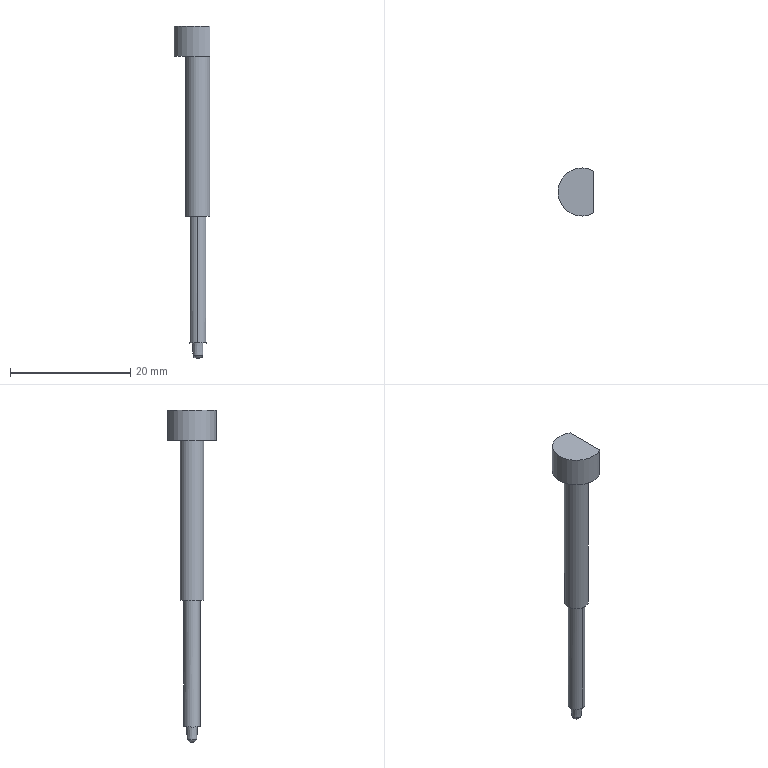Part | NX | features solid 2 | 1 solid | 12 faces | box 6 x 8 x 55.164 mm | volume 670.32 mm3 | plane 5 | cylinder 4 | cone 2 | torus 1 | commonest cylinder face diameters 2.785 x2 4 x1 8 x1
STEP:
#1=CARTESIAN_POINT('',(2.,37.688,65.5));
#2=VERTEX_POINT('',#1);
#3=CARTESIAN_POINT('',(0.,37.688,65.5));
#4=DIRECTION('',(0.,0.,-1.));
#5=DIRECTION('',(-1.,0.,0.));
#6=AXIS2_PLACEMENT_3D('',#3,#4,#5);
#7=CIRCLE('',#6,2.);
#8=EDGE_CURVE('',#2,#2,#7,.F.);
#9=ORIENTED_EDGE('',*,*,#8,.F.);
#10=EDGE_LOOP('',(#9));
#11=FACE_BOUND('',#10,.T.);
#12=CARTESIAN_POINT('',(-2.,37.688,38.875));
#13=VERTEX_POINT('',#12);
#14=CARTESIAN_POINT('',(0.,37.688,38.875));
#15=DIRECTION('',(0.,0.,-1.));
#16=DIRECTION('',(-1.,0.,0.));
#17=AXIS2_PLACEMENT_3D('',#14,#15,#16);
#18=CIRCLE('',#17,2.);
#19=EDGE_CURVE('',#13,#13,#18,.F.);
#20=ORIENTED_EDGE('',*,*,#19,.T.);
#21=EDGE_LOOP('',(#20));
#22=FACE_BOUND('',#21,.T.);
#23=CARTESIAN_POINT('',(0.,37.688,117.875));
#24=DIRECTION('',(0.,0.,-1.));
#25=DIRECTION('',(-1.,0.,0.));
#26=AXIS2_PLACEMENT_3D('',#23,#24,#25);
#27=CYLINDRICAL_SURFACE('',#26,2.);
#28=ADVANCED_FACE('',(#11,#22),#27,.T.);
#29=CARTESIAN_POINT('',(2.,34.223,65.5));
#30=VERTEX_POINT('',#29);
#31=CARTESIAN_POINT('',(2.,41.152,65.5));
#32=VERTEX_POINT('',#31);
#33=CARTESIAN_POINT('',(0.,37.688,65.5));
#34=DIRECTION('',(0.,0.,-1.));
#35=DIRECTION('',(-1.,0.,0.));
#36=AXIS2_PLACEMENT_3D('',#33,#34,#35);
#37=CIRCLE('',#36,4.);
#38=EDGE_CURVE('',#30,#32,#37,.T.);
#39=ORIENTED_EDGE('',*,*,#38,.F.);
#40=CARTESIAN_POINT('',(2.,34.223,70.5));
#41=VERTEX_POINT('',#40);
#42=CARTESIAN_POINT('',(2.,34.223,66.5));
#43=DIRECTION('',(0.,0.,1.));
#44=VECTOR('',#43,1000.);
#45=LINE('',#42,#44);
#46=EDGE_CURVE('',#41,#30,#45,.F.);
#47=ORIENTED_EDGE('',*,*,#46,.F.);
#48=CARTESIAN_POINT('',(2.,41.152,70.5));
#49=VERTEX_POINT('',#48);
#50=CARTESIAN_POINT('',(0.,37.688,70.5));
#51=DIRECTION('',(0.,0.,1.));
#52=DIRECTION('',(1.,0.,0.));
#53=AXIS2_PLACEMENT_3D('',#50,#51,#52);
#54=CIRCLE('',#53,4.);
#55=EDGE_CURVE('',#41,#49,#54,.F.);
#56=ORIENTED_EDGE('',*,*,#55,.T.);
#57=CARTESIAN_POINT('',(2.,41.152,66.5));
#58=DIRECTION('',(0.,0.,1.));
#59=VECTOR('',#58,1000.);
#60=LINE('',#57,#59);
#61=EDGE_CURVE('',#32,#49,#60,.T.);
#62=ORIENTED_EDGE('',*,*,#61,.F.);
#63=EDGE_LOOP('',(#39,#47,#56,#62));
#64=FACE_BOUND('',#63,.T.);
#65=CARTESIAN_POINT('',(0.,37.688,66.5));
#66=DIRECTION('',(0.,0.,1.));
#67=DIRECTION('',(1.,0.,0.));
#68=AXIS2_PLACEMENT_3D('',#65,#66,#67);
#69=CYLINDRICAL_SURFACE('',#68,4.);
#70=ADVANCED_FACE('',(#64),#69,.T.);
#71=CARTESIAN_POINT('',(2.,37.688,65.5));
#72=DIRECTION('',(0.,-1.,0.));
#73=VECTOR('',#72,1000.);
#74=LINE('',#71,#73);
#75=EDGE_CURVE('',#2,#32,#74,.F.);
#76=ORIENTED_EDGE('',*,*,#75,.F.);
#77=ORIENTED_EDGE('',*,*,#8,.T.);
#78=CARTESIAN_POINT('',(2.,37.688,65.5));
#79=DIRECTION('',(0.,-1.,0.));
#80=VECTOR('',#79,1000.);
#81=LINE('',#78,#80);
#82=EDGE_CURVE('',#30,#2,#81,.F.);
#83=ORIENTED_EDGE('',*,*,#82,.F.);
#84=ORIENTED_EDGE('',*,*,#38,.T.);
#85=EDGE_LOOP('',(#76,#77,#83,#84));
#86=FACE_BOUND('',#85,.T.);
#87=CARTESIAN_POINT('',(0.,37.688,65.5));
#88=DIRECTION('',(0.,0.,-1.));
#89=DIRECTION('',(-1.,0.,0.));
#90=AXIS2_PLACEMENT_3D('',#87,#88,#89);
#91=PLANE('',#90);
#92=ADVANCED_FACE('',(#86),#91,.T.);
#93=CARTESIAN_POINT('',(2.,0.,70.5));
#94=DIRECTION('',(0.,1.,0.));
#95=VECTOR('',#94,1000.);
#96=LINE('',#93,#95);
#97=EDGE_CURVE('',#49,#41,#96,.F.);
#98=ORIENTED_EDGE('',*,*,#97,.F.);
#99=ORIENTED_EDGE('',*,*,#55,.F.);
#100=EDGE_LOOP('',(#98,#99));
#101=FACE_BOUND('',#100,.T.);
#102=CARTESIAN_POINT('',(0.,0.,70.5));
#103=DIRECTION('',(0.,0.,1.));
#104=DIRECTION('',(1.,0.,0.));
#105=AXIS2_PLACEMENT_3D('',#102,#103,#104);
#106=PLANE('',#105);
#107=ADVANCED_FACE('',(#101),#106,.T.);
#108=CARTESIAN_POINT('',(0.,36.295,17.916));
#109=VERTEX_POINT('',#108);
#110=CARTESIAN_POINT('',(0.,39.08,17.94));
#111=VERTEX_POINT('',#110);
#112=CARTESIAN_POINT('',(0.,36.295,17.916));
#113=CARTESIAN_POINT('',(0.3656,36.295,17.916));
#114=CARTESIAN_POINT('',(1.09,36.596,17.866));
#115=CARTESIAN_POINT('',(1.544,37.687,17.795));
#116=CARTESIAN_POINT('',(1.09,38.779,17.885));
#117=CARTESIAN_POINT('',(0.3667,39.08,17.94));
#118=CARTESIAN_POINT('',(0.,39.08,17.94));
#119=B_SPLINE_CURVE_WITH_KNOTS('',3,(#112,#113,#114,#115,#116,#117,#118),.UNSPECIFIED.,.F.,.F.,(4,1,1,1,4),(0.00007924,0.001169,0.002259,0.003349,0.004439),.UNSPECIFIED.);
#120=EDGE_CURVE('',#109,#111,#119,.T.);
#121=ORIENTED_EDGE('',*,*,#120,.T.);
#122=CARTESIAN_POINT('',(0.,39.08,38.875));
#123=VERTEX_POINT('',#122);
#124=CARTESIAN_POINT('',(0.,39.08,38.875));
#125=DIRECTION('',(0.,0.,-1.));
#126=VECTOR('',#125,1000.);
#127=LINE('',#124,#126);
#128=EDGE_CURVE('',#111,#123,#127,.F.);
#129=ORIENTED_EDGE('',*,*,#128,.T.);
#130=CARTESIAN_POINT('',(0.,36.295,38.875));
#131=VERTEX_POINT('',#130);
#132=CARTESIAN_POINT('',(0.,37.688,38.875));
#133=DIRECTION('',(0.,0.,1.));
#134=DIRECTION('',(0.,-1.,0.));
#135=AXIS2_PLACEMENT_3D('',#132,#133,#134);
#136=CIRCLE('',#135,1.393);
#137=EDGE_CURVE('',#123,#131,#136,.F.);
#138=ORIENTED_EDGE('',*,*,#137,.T.);
#139=CARTESIAN_POINT('',(0.,36.295,38.875));
#140=DIRECTION('',(0.,0.,-1.));
#141=VECTOR('',#140,1000.);
#142=LINE('',#139,#141);
#143=EDGE_CURVE('',#131,#109,#142,.T.);
#144=ORIENTED_EDGE('',*,*,#143,.T.);
#145=EDGE_LOOP('',(#121,#129,#138,#144));
#146=FACE_BOUND('',#145,.T.);
#147=CARTESIAN_POINT('',(0.,37.688,38.875));
#148=DIRECTION('',(0.,0.,1.));
#149=DIRECTION('',(0.,1.,0.));
#150=AXIS2_PLACEMENT_3D('',#147,#148,#149);
#151=CYLINDRICAL_SURFACE('',#150,1.393);
#152=ADVANCED_FACE('',(#146),#151,.T.);
#153=CARTESIAN_POINT('',(0.,39.08,17.94));
#154=CARTESIAN_POINT('',(-0.3656,39.08,17.94));
#155=CARTESIAN_POINT('',(-1.089,38.779,17.885));
#156=CARTESIAN_POINT('',(-1.544,37.69,17.795));
#157=CARTESIAN_POINT('',(-1.091,36.596,17.866));
#158=CARTESIAN_POINT('',(-0.3667,36.295,17.916));
#159=CARTESIAN_POINT('',(0.,36.295,17.916));
#160=B_SPLINE_CURVE_WITH_KNOTS('',3,(#153,#154,#155,#156,#157,#158,#159),.UNSPECIFIED.,.F.,.F.,(4,1,1,1,4),(0.00007934,0.001169,0.002259,0.003349,0.004439),.UNSPECIFIED.);
#161=EDGE_CURVE('',#111,#109,#160,.T.);
#162=ORIENTED_EDGE('',*,*,#161,.T.);
#163=ORIENTED_EDGE('',*,*,#143,.F.);
#164=CARTESIAN_POINT('',(0.,37.688,38.875));
#165=DIRECTION('',(0.,0.,1.));
#166=DIRECTION('',(0.,1.,0.));
#167=AXIS2_PLACEMENT_3D('',#164,#165,#166);
#168=CIRCLE('',#167,1.393);
#169=EDGE_CURVE('',#131,#123,#168,.F.);
#170=ORIENTED_EDGE('',*,*,#169,.T.);
#171=ORIENTED_EDGE('',*,*,#128,.F.);
#172=EDGE_LOOP('',(#162,#163,#170,#171));
#173=FACE_BOUND('',#172,.T.);
#174=CARTESIAN_POINT('',(0.,37.688,38.875));
#175=DIRECTION('',(0.,0.,1.));
#176=DIRECTION('',(0.,1.,0.));
#177=AXIS2_PLACEMENT_3D('',#174,#175,#176);
#178=CYLINDRICAL_SURFACE('',#177,1.393);
#179=ADVANCED_FACE('',(#173),#178,.T.);
#180=ORIENTED_EDGE('',*,*,#19,.F.);
#181=EDGE_LOOP('',(#180));
#182=FACE_BOUND('',#181,.T.);
#183=ORIENTED_EDGE('',*,*,#169,.F.);
#184=ORIENTED_EDGE('',*,*,#137,.F.);
#185=EDGE_LOOP('',(#183,#184));
#186=FACE_BOUND('',#185,.T.);
#187=CARTESIAN_POINT('',(0.,37.688,38.875));
#188=DIRECTION('',(0.,0.,-1.));
#189=DIRECTION('',(0.,-1.,0.));
#190=AXIS2_PLACEMENT_3D('',#187,#188,#189);
#191=PLANE('',#190);
#192=ADVANCED_FACE('',(#182,#186),#191,.T.);
#193=CARTESIAN_POINT('',(-0.3071,37.688,15.336));
#194=VERTEX_POINT('',#193);
#195=CARTESIAN_POINT('',(0.,37.688,15.336));
#196=DIRECTION('',(0.,0.,-1.));
#197=DIRECTION('',(-1.,0.,0.));
#198=AXIS2_PLACEMENT_3D('',#195,#196,#197);
#199=CIRCLE('',#198,0.3071);
#200=EDGE_CURVE('',#194,#194,#199,.T.);
#201=ORIENTED_EDGE('',*,*,#200,.T.);
#202=EDGE_LOOP('',(#201));
#203=FACE_BOUND('',#202,.T.);
#204=CARTESIAN_POINT('',(0.,37.688,15.336));
#205=DIRECTION('',(0.,0.,-1.));
#206=DIRECTION('',(-1.,0.,0.));
#207=AXIS2_PLACEMENT_3D('',#204,#205,#206);
#208=PLANE('',#207);
#209=ADVANCED_FACE('',(#203),#208,.T.);
#210=CARTESIAN_POINT('',(-0.8064,37.688,15.81));
#211=VERTEX_POINT('',#210);
#212=CARTESIAN_POINT('',(0.,37.688,15.81));
#213=DIRECTION('',(0.,0.,-1.));
#214=DIRECTION('',(-1.,0.,0.));
#215=AXIS2_PLACEMENT_3D('',#212,#213,#214);
#216=CIRCLE('',#215,0.8064);
#217=EDGE_CURVE('',#211,#211,#216,.F.);
#218=ORIENTED_EDGE('',*,*,#217,.T.);
#219=EDGE_LOOP('',(#218));
#220=FACE_BOUND('',#219,.T.);
#221=CARTESIAN_POINT('',(-0.9135,37.634,17.882));
#222=VERTEX_POINT('',#221);
#223=CARTESIAN_POINT('',(-0.7599,38.361,17.907));
#224=CARTESIAN_POINT('',(-1.012,37.629,17.871));
#225=CARTESIAN_POINT('',(-0.6747,36.928,17.902));
#226=CARTESIAN_POINT('',(0.05937,36.673,17.93));
#227=CARTESIAN_POINT('',(0.7563,37.011,17.895));
#228=CARTESIAN_POINT('',(1.107,38.004,17.865));
#229=CARTESIAN_POINT('',(0.1856,38.828,17.962));
#230=CARTESIAN_POINT('',(-0.7599,38.361,17.907));
#231=CARTESIAN_POINT('',(-1.012,37.629,17.871));
#232=CARTESIAN_POINT('',(-0.6747,36.928,17.902));
#233=B_SPLINE_CURVE_WITH_KNOTS('',3,(#223,#224,#225,#226,#227,#228,#229,#230,#231,#232),.UNSPECIFIED.,.T.,.F.,(1,1,1,1,1,1,1,1,1,1,1,1,1,1),(-0.002866,-0.001433,-0.0007165,0.,0.0007165,0.001433,0.00215,0.002866,0.004299,0.005016,0.005732,0.006449,0.007165,0.007882),.UNSPECIFIED.);
#234=EDGE_CURVE('',#222,#222,#233,.T.);
#235=ORIENTED_EDGE('',*,*,#234,.F.);
#236=EDGE_LOOP('',(#235));
#237=FACE_BOUND('',#236,.T.);
#238=CARTESIAN_POINT('',(0.,37.688,15.336));
#239=DIRECTION('',(0.,0.,1.));
#240=DIRECTION('',(-1.,0.,0.));
#241=AXIS2_PLACEMENT_3D('',#238,#239,#240);
#242=CONICAL_SURFACE('',#241,0.7816,0.05236);
#243=ADVANCED_FACE('',(#220,#237),#242,.T.);
#244=ORIENTED_EDGE('',*,*,#234,.T.);
#245=EDGE_LOOP('',(#244));
#246=FACE_BOUND('',#245,.T.);
#247=ORIENTED_EDGE('',*,*,#120,.F.);
#248=ORIENTED_EDGE('',*,*,#161,.F.);
#249=EDGE_LOOP('',(#247,#248));
#250=FACE_BOUND('',#249,.T.);
#251=CARTESIAN_POINT('',(0.,48.993,8.725));
#252=DIRECTION('',(0.,1.,0.));
#253=DIRECTION('',(0.,0.,-1.));
#254=AXIS2_PLACEMENT_3D('',#251,#252,#253);
#255=CONICAL_SURFACE('',#254,9.301,0.008727);
#256=ADVANCED_FACE('',(#246,#250),#255,.F.);
#257=ORIENTED_EDGE('',*,*,#82,.T.);
#258=ORIENTED_EDGE('',*,*,#75,.T.);
#259=ORIENTED_EDGE('',*,*,#61,.T.);
#260=ORIENTED_EDGE('',*,*,#97,.T.);
#261=ORIENTED_EDGE('',*,*,#46,.T.);
#262=EDGE_LOOP('',(#257,#258,#259,#260,#261));
#263=FACE_BOUND('',#262,.T.);
#264=CARTESIAN_POINT('',(2.,37.688,65.5));
#265=DIRECTION('',(1.,0.,0.));
#266=DIRECTION('',(0.,0.,-1.));
#267=AXIS2_PLACEMENT_3D('',#264,#265,#266);
#268=PLANE('',#267);
#269=ADVANCED_FACE('',(#263),#268,.T.);
#270=ORIENTED_EDGE('',*,*,#200,.F.);
#271=EDGE_LOOP('',(#270));
#272=FACE_BOUND('',#271,.T.);
#273=ORIENTED_EDGE('',*,*,#217,.F.);
#274=EDGE_LOOP('',(#273));
#275=FACE_BOUND('',#274,.T.);
#276=CARTESIAN_POINT('',(0.,37.688,15.836));
#277=DIRECTION('',(0.,0.,-1.));
#278=DIRECTION('',(-1.,0.,0.));
#279=AXIS2_PLACEMENT_3D('',#276,#277,#278);
#280=DEGENERATE_TOROIDAL_SURFACE('',#279,0.3071,0.5,.T.);
#281=ADVANCED_FACE('',(#272,#275),#280,.T.);
#282=CLOSED_SHELL('',(#28,#70,#92,#107,#152,#179,#192,#209,#243,#256,#269,#281));
#283=MANIFOLD_SOLID_BREP('',#282);
#284=(LENGTH_UNIT()NAMED_UNIT(*)SI_UNIT(.MILLI.,.METRE.));
#285=UNCERTAINTY_MEASURE_WITH_UNIT(LENGTH_MEASURE(0.0508),#284,'','');
#286=(NAMED_UNIT(*)PLANE_ANGLE_UNIT()SI_UNIT($,.RADIAN.));
#287=(NAMED_UNIT(*)SI_UNIT($,.STERADIAN.)SOLID_ANGLE_UNIT());
#288=(GEOMETRIC_REPRESENTATION_CONTEXT(3)GLOBAL_UNCERTAINTY_ASSIGNED_CONTEXT((#285))GLOBAL_UNIT_ASSIGNED_CONTEXT((#284,#286,#287))REPRESENTATION_CONTEXT('',''));
#289=ADVANCED_BREP_SHAPE_REPRESENTATION('',(#283),#288);